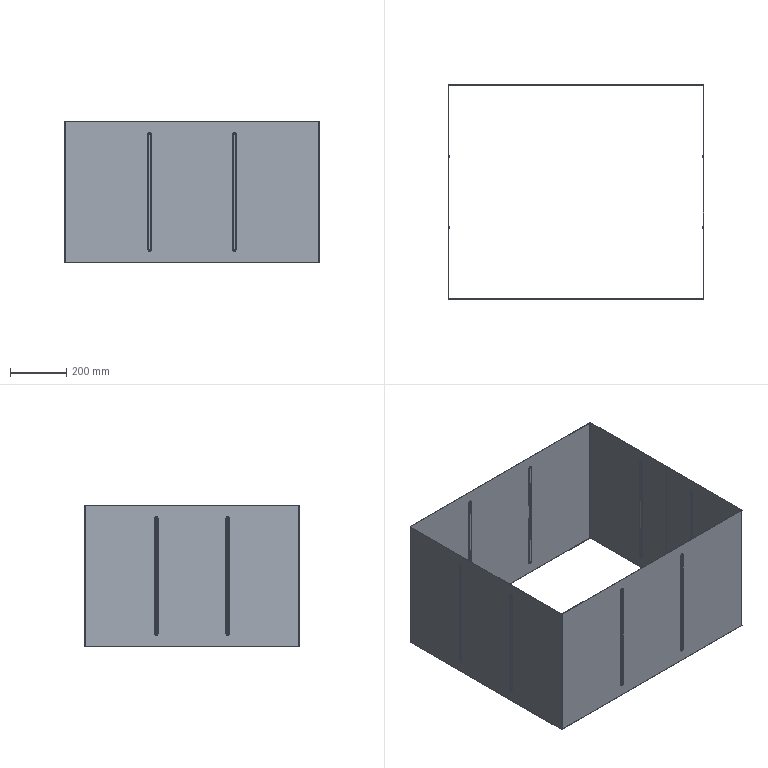Part | STEP file | 750078481 | 1 solid | 152 faces | box 906 x 762 x 500 mm | volume 2504428 mm3 | spline 78 | cylinder 60 | plane 14 | commonest cylinder face diameters 6 x30 9 x26 3 x4